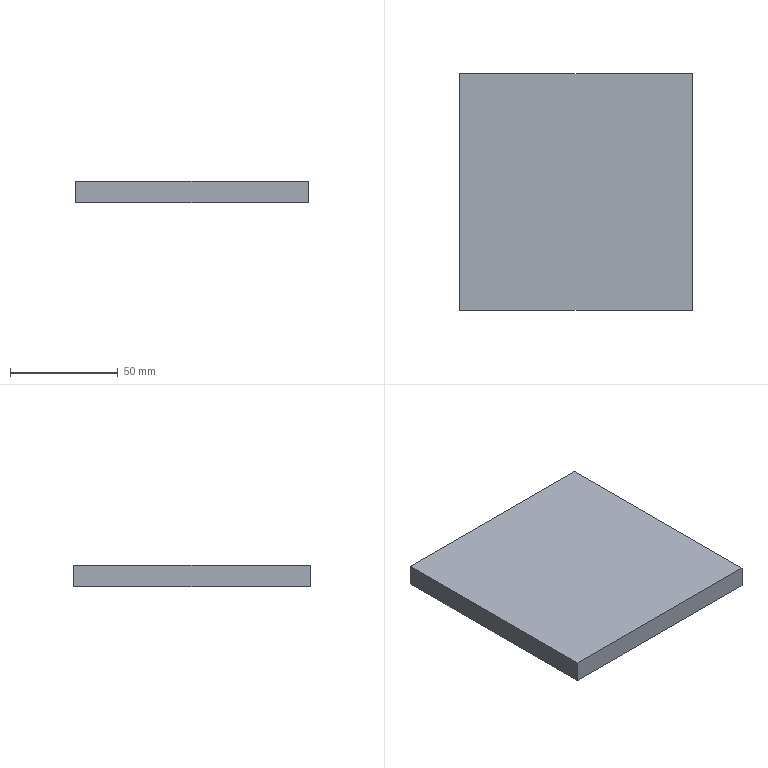Part | SolidWorks | features Extrusion 1 | 1 solid | 6 faces | box 108 x 110 x 10 mm | volume 118800 mm3 | plane 6
STEP:
#1=CARTESIAN_POINT('',(54.,-55.,-5.));
#2=VERTEX_POINT('',#1);
#3=CARTESIAN_POINT('',(54.,55.,-5.));
#4=VERTEX_POINT('',#3);
#5=CARTESIAN_POINT('',(54.,-55.,-5.));
#6=DIRECTION('',(0.,1.,0.));
#7=VECTOR('',#6,1000.);
#8=LINE('',#5,#7);
#9=EDGE_CURVE('',#2,#4,#8,.T.);
#10=ORIENTED_EDGE('',*,*,#9,.T.);
#11=CARTESIAN_POINT('',(54.,55.,5.));
#12=VERTEX_POINT('',#11);
#13=CARTESIAN_POINT('',(54.,55.,5.));
#14=DIRECTION('',(0.,0.,-1.));
#15=VECTOR('',#14,1000.);
#16=LINE('',#13,#15);
#17=EDGE_CURVE('',#12,#4,#16,.T.);
#18=ORIENTED_EDGE('',*,*,#17,.F.);
#19=CARTESIAN_POINT('',(54.,-55.,5.));
#20=VERTEX_POINT('',#19);
#21=CARTESIAN_POINT('',(54.,-55.,5.));
#22=DIRECTION('',(0.,1.,0.));
#23=VECTOR('',#22,1000.);
#24=LINE('',#21,#23);
#25=EDGE_CURVE('',#20,#12,#24,.T.);
#26=ORIENTED_EDGE('',*,*,#25,.F.);
#27=CARTESIAN_POINT('',(54.,-55.,5.));
#28=DIRECTION('',(0.,0.,-1.));
#29=VECTOR('',#28,1000.);
#30=LINE('',#27,#29);
#31=EDGE_CURVE('',#20,#2,#30,.T.);
#32=ORIENTED_EDGE('',*,*,#31,.T.);
#33=EDGE_LOOP('',(#10,#18,#26,#32));
#34=FACE_OUTER_BOUND('',#33,.T.);
#35=CARTESIAN_POINT('',(54.,-55.,5.));
#36=DIRECTION('',(-1.,0.,0.));
#37=DIRECTION('',(0.,0.,1.));
#38=AXIS2_PLACEMENT_3D('',#35,#36,#37);
#39=PLANE('',#38);
#40=ADVANCED_FACE('',(#34),#39,.F.);
#41=CARTESIAN_POINT('',(-54.,55.,-5.));
#42=VERTEX_POINT('',#41);
#43=CARTESIAN_POINT('',(-54.,55.,-5.));
#44=DIRECTION('',(-1.,0.,0.));
#45=VECTOR('',#44,1000.);
#46=LINE('',#43,#45);
#47=EDGE_CURVE('',#4,#42,#46,.T.);
#48=ORIENTED_EDGE('',*,*,#47,.T.);
#49=CARTESIAN_POINT('',(-54.,55.,5.));
#50=VERTEX_POINT('',#49);
#51=CARTESIAN_POINT('',(-54.,55.,5.));
#52=DIRECTION('',(0.,0.,-1.));
#53=VECTOR('',#52,1000.);
#54=LINE('',#51,#53);
#55=EDGE_CURVE('',#50,#42,#54,.T.);
#56=ORIENTED_EDGE('',*,*,#55,.F.);
#57=CARTESIAN_POINT('',(-54.,55.,5.));
#58=DIRECTION('',(-1.,0.,0.));
#59=VECTOR('',#58,1000.);
#60=LINE('',#57,#59);
#61=EDGE_CURVE('',#12,#50,#60,.T.);
#62=ORIENTED_EDGE('',*,*,#61,.F.);
#63=ORIENTED_EDGE('',*,*,#17,.T.);
#64=EDGE_LOOP('',(#48,#56,#62,#63));
#65=FACE_OUTER_BOUND('',#64,.T.);
#66=CARTESIAN_POINT('',(-54.,55.,5.));
#67=DIRECTION('',(0.,-1.,0.));
#68=DIRECTION('',(0.,0.,-1.));
#69=AXIS2_PLACEMENT_3D('',#66,#67,#68);
#70=PLANE('',#69);
#71=ADVANCED_FACE('',(#65),#70,.F.);
#72=CARTESIAN_POINT('',(-54.,-55.,-5.));
#73=VERTEX_POINT('',#72);
#74=CARTESIAN_POINT('',(-54.,-55.,-5.));
#75=DIRECTION('',(0.,-1.,0.));
#76=VECTOR('',#75,1000.);
#77=LINE('',#74,#76);
#78=EDGE_CURVE('',#42,#73,#77,.T.);
#79=ORIENTED_EDGE('',*,*,#78,.T.);
#80=CARTESIAN_POINT('',(-54.,-55.,5.));
#81=VERTEX_POINT('',#80);
#82=CARTESIAN_POINT('',(-54.,-55.,5.));
#83=DIRECTION('',(0.,0.,-1.));
#84=VECTOR('',#83,1000.);
#85=LINE('',#82,#84);
#86=EDGE_CURVE('',#81,#73,#85,.T.);
#87=ORIENTED_EDGE('',*,*,#86,.F.);
#88=CARTESIAN_POINT('',(-54.,-55.,5.));
#89=DIRECTION('',(0.,-1.,0.));
#90=VECTOR('',#89,1000.);
#91=LINE('',#88,#90);
#92=EDGE_CURVE('',#50,#81,#91,.T.);
#93=ORIENTED_EDGE('',*,*,#92,.F.);
#94=ORIENTED_EDGE('',*,*,#55,.T.);
#95=EDGE_LOOP('',(#79,#87,#93,#94));
#96=FACE_OUTER_BOUND('',#95,.T.);
#97=CARTESIAN_POINT('',(-54.,-55.,5.));
#98=DIRECTION('',(1.,0.,0.));
#99=DIRECTION('',(0.,0.,-1.));
#100=AXIS2_PLACEMENT_3D('',#97,#98,#99);
#101=PLANE('',#100);
#102=ADVANCED_FACE('',(#96),#101,.F.);
#103=CARTESIAN_POINT('',(-54.,-55.,-5.));
#104=DIRECTION('',(1.,0.,0.));
#105=VECTOR('',#104,1000.);
#106=LINE('',#103,#105);
#107=EDGE_CURVE('',#73,#2,#106,.T.);
#108=ORIENTED_EDGE('',*,*,#107,.T.);
#109=ORIENTED_EDGE('',*,*,#31,.F.);
#110=CARTESIAN_POINT('',(-54.,-55.,5.));
#111=DIRECTION('',(1.,0.,0.));
#112=VECTOR('',#111,1000.);
#113=LINE('',#110,#112);
#114=EDGE_CURVE('',#81,#20,#113,.T.);
#115=ORIENTED_EDGE('',*,*,#114,.F.);
#116=ORIENTED_EDGE('',*,*,#86,.T.);
#117=EDGE_LOOP('',(#108,#109,#115,#116));
#118=FACE_OUTER_BOUND('',#117,.T.);
#119=CARTESIAN_POINT('',(-54.,-55.,5.));
#120=DIRECTION('',(0.,1.,0.));
#121=DIRECTION('',(0.,0.,1.));
#122=AXIS2_PLACEMENT_3D('',#119,#120,#121);
#123=PLANE('',#122);
#124=ADVANCED_FACE('',(#118),#123,.F.);
#125=ORIENTED_EDGE('',*,*,#25,.T.);
#126=ORIENTED_EDGE('',*,*,#61,.T.);
#127=ORIENTED_EDGE('',*,*,#92,.T.);
#128=ORIENTED_EDGE('',*,*,#114,.T.);
#129=EDGE_LOOP('',(#125,#126,#127,#128));
#130=FACE_OUTER_BOUND('',#129,.T.);
#131=CARTESIAN_POINT('',(0.,0.,5.));
#132=DIRECTION('',(0.,0.,-1.));
#133=DIRECTION('',(-1.,0.,0.));
#134=AXIS2_PLACEMENT_3D('',#131,#132,#133);
#135=PLANE('',#134);
#136=ADVANCED_FACE('',(#130),#135,.F.);
#137=ORIENTED_EDGE('',*,*,#9,.F.);
#138=ORIENTED_EDGE('',*,*,#107,.F.);
#139=ORIENTED_EDGE('',*,*,#78,.F.);
#140=ORIENTED_EDGE('',*,*,#47,.F.);
#141=EDGE_LOOP('',(#137,#138,#139,#140));
#142=FACE_OUTER_BOUND('',#141,.T.);
#143=CARTESIAN_POINT('',(0.,0.,-5.));
#144=DIRECTION('',(0.,0.,-1.));
#145=DIRECTION('',(-1.,0.,0.));
#146=AXIS2_PLACEMENT_3D('',#143,#144,#145);
#147=PLANE('',#146);
#148=ADVANCED_FACE('',(#142),#147,.T.);
#149=CLOSED_SHELL('',(#40,#71,#102,#124,#136,#148));
#150=MANIFOLD_SOLID_BREP('',#149);
#151=CARTESIAN_POINT('',(0.,0.,0.));
#152=DIRECTION('',(0.,0.,1.));
#153=DIRECTION('',(1.,0.,0.));
#154=AXIS2_PLACEMENT_3D('',#151,#152,#153);
#155=(LENGTH_UNIT()NAMED_UNIT(*)SI_UNIT(.MILLI.,.METRE.));
#156=UNCERTAINTY_MEASURE_WITH_UNIT(LENGTH_MEASURE(0.00001),#155,'','');
#157=(NAMED_UNIT(*)PLANE_ANGLE_UNIT()SI_UNIT($,.RADIAN.));
#158=(NAMED_UNIT(*)SI_UNIT($,.STERADIAN.)SOLID_ANGLE_UNIT());
#159=(GEOMETRIC_REPRESENTATION_CONTEXT(3)GLOBAL_UNCERTAINTY_ASSIGNED_CONTEXT((#156))GLOBAL_UNIT_ASSIGNED_CONTEXT((#155,#157,#158))REPRESENTATION_CONTEXT('',''));
#160=ADVANCED_BREP_SHAPE_REPRESENTATION('',(#150,#154),#159);